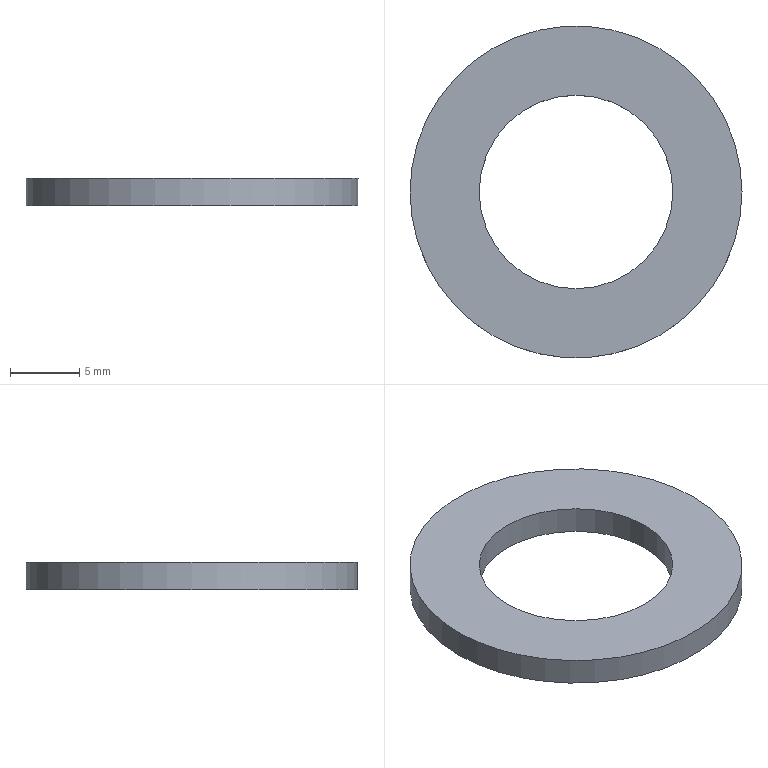Part | NX | features solid 2 | 1 solid | 4 faces | box 24 x 24 x 2 mm | volume 596.903 mm3 | plane 2 | cylinder 2 | commonest cylinder face diameters 14 x1 24 x1
STEP:
#1=CARTESIAN_POINT('',(-22.,99.3,73.5));
#2=VERTEX_POINT('',#1);
#3=CARTESIAN_POINT('',(-15.,99.3,73.5));
#4=DIRECTION('',(-0.000000009,0.,-1.));
#5=DIRECTION('',(-1.,0.,0.000000009));
#6=AXIS2_PLACEMENT_3D('',#3,#4,#5);
#7=CIRCLE('',#6,7.);
#8=EDGE_CURVE('',#2,#2,#7,.T.);
#9=ORIENTED_EDGE('',*,*,#8,.F.);
#10=EDGE_LOOP('',(#9));
#11=FACE_BOUND('',#10,.T.);
#12=CARTESIAN_POINT('',(-27.,99.3,73.5));
#13=VERTEX_POINT('',#12);
#14=CARTESIAN_POINT('',(-15.,99.3,73.5));
#15=DIRECTION('',(0.000000009,0.,1.));
#16=DIRECTION('',(-1.,-0.000000075,0.000000009));
#17=AXIS2_PLACEMENT_3D('',#14,#15,#16);
#18=CIRCLE('',#17,12.);
#19=EDGE_CURVE('',#13,#13,#18,.T.);
#20=ORIENTED_EDGE('',*,*,#19,.F.);
#21=EDGE_LOOP('',(#20));
#22=FACE_BOUND('',#21,.T.);
#23=CARTESIAN_POINT('',(-15.,99.3,73.5));
#24=DIRECTION('',(-0.000000009,0.,-1.));
#25=DIRECTION('',(-1.,0.,0.000000009));
#26=AXIS2_PLACEMENT_3D('',#23,#24,#25);
#27=PLANE('',#26);
#28=ADVANCED_FACE('',(#11,#22),#27,.T.);
#29=CARTESIAN_POINT('',(-8.,99.3,75.5));
#30=VERTEX_POINT('',#29);
#31=CARTESIAN_POINT('',(-15.,99.3,75.5));
#32=DIRECTION('',(0.000000009,0.,1.));
#33=DIRECTION('',(1.,0.,-0.000000009));
#34=AXIS2_PLACEMENT_3D('',#31,#32,#33);
#35=CIRCLE('',#34,7.);
#36=EDGE_CURVE('',#30,#30,#35,.T.);
#37=ORIENTED_EDGE('',*,*,#36,.F.);
#38=EDGE_LOOP('',(#37));
#39=FACE_BOUND('',#38,.T.);
#40=CARTESIAN_POINT('',(-27.,99.3,75.5));
#41=VERTEX_POINT('',#40);
#42=CARTESIAN_POINT('',(-15.,99.3,75.5));
#43=DIRECTION('',(-0.000000009,0.,-1.));
#44=DIRECTION('',(-1.,-0.000000075,0.000000009));
#45=AXIS2_PLACEMENT_3D('',#42,#43,#44);
#46=CIRCLE('',#45,12.);
#47=EDGE_CURVE('',#41,#41,#46,.T.);
#48=ORIENTED_EDGE('',*,*,#47,.F.);
#49=EDGE_LOOP('',(#48));
#50=FACE_BOUND('',#49,.T.);
#51=CARTESIAN_POINT('',(-15.,99.3,75.5));
#52=DIRECTION('',(0.000000009,0.,1.));
#53=DIRECTION('',(1.,0.,-0.000000009));
#54=AXIS2_PLACEMENT_3D('',#51,#52,#53);
#55=PLANE('',#54);
#56=ADVANCED_FACE('',(#39,#50),#55,.T.);
#57=ORIENTED_EDGE('',*,*,#19,.T.);
#58=EDGE_LOOP('',(#57));
#59=FACE_BOUND('',#58,.T.);
#60=ORIENTED_EDGE('',*,*,#47,.T.);
#61=EDGE_LOOP('',(#60));
#62=FACE_BOUND('',#61,.T.);
#63=CARTESIAN_POINT('',(-15.,99.3,75.5));
#64=DIRECTION('',(-0.000000009,0.,-1.));
#65=DIRECTION('',(-1.,-0.000000075,0.000000009));
#66=AXIS2_PLACEMENT_3D('',#63,#64,#65);
#67=CYLINDRICAL_SURFACE('',#66,12.);
#68=ADVANCED_FACE('',(#59,#62),#67,.T.);
#69=ORIENTED_EDGE('',*,*,#8,.T.);
#70=EDGE_LOOP('',(#69));
#71=FACE_BOUND('',#70,.T.);
#72=ORIENTED_EDGE('',*,*,#36,.T.);
#73=EDGE_LOOP('',(#72));
#74=FACE_BOUND('',#73,.T.);
#75=CARTESIAN_POINT('',(-15.,99.3,22.5));
#76=DIRECTION('',(-0.000000009,0.,-1.));
#77=DIRECTION('',(0.,1.,0.));
#78=AXIS2_PLACEMENT_3D('',#75,#76,#77);
#79=CYLINDRICAL_SURFACE('',#78,7.);
#80=ADVANCED_FACE('',(#71,#74),#79,.F.);
#81=CLOSED_SHELL('',(#28,#56,#68,#80));
#82=MANIFOLD_SOLID_BREP('',#81);
#83=(LENGTH_UNIT()NAMED_UNIT(*)SI_UNIT(.MILLI.,.METRE.));
#84=UNCERTAINTY_MEASURE_WITH_UNIT(LENGTH_MEASURE(0.00001),#83,'','');
#85=(NAMED_UNIT(*)PLANE_ANGLE_UNIT()SI_UNIT($,.RADIAN.));
#86=(NAMED_UNIT(*)SI_UNIT($,.STERADIAN.)SOLID_ANGLE_UNIT());
#87=(GEOMETRIC_REPRESENTATION_CONTEXT(3)GLOBAL_UNCERTAINTY_ASSIGNED_CONTEXT((#84))GLOBAL_UNIT_ASSIGNED_CONTEXT((#83,#85,#86))REPRESENTATION_CONTEXT('',''));
#88=ADVANCED_BREP_SHAPE_REPRESENTATION('',(#82),#87);